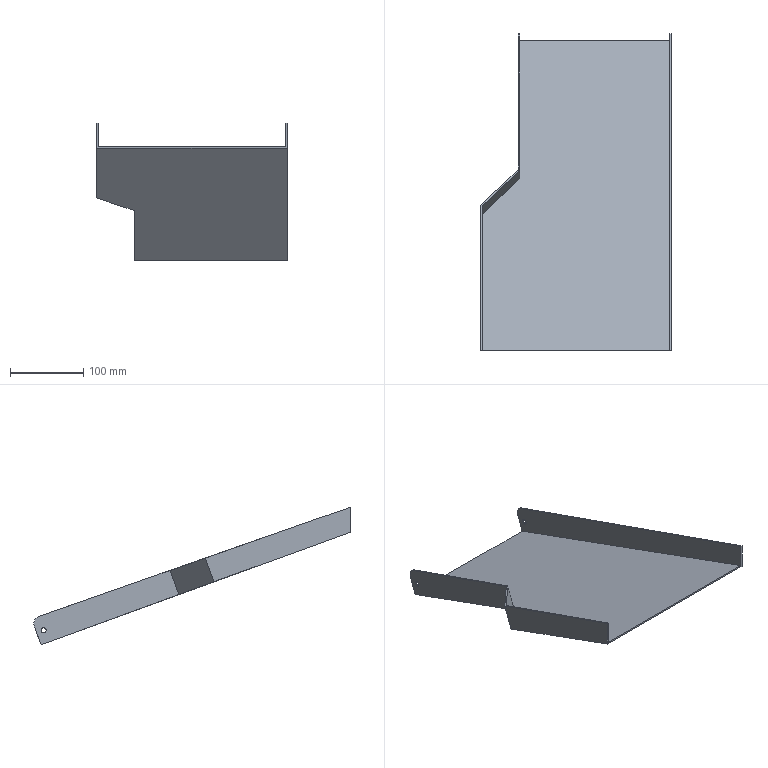Part | NX | features HB 2 | 1 solid | 18 faces | box 260 x 431.386 x 187.459 mm | volume 271044 mm3 | plane 14 | cylinder 4 | commonest cylinder face diameters 7 x2 20 x2
STEP:
#1=CARTESIAN_POINT('',(3672.,269.,-204.418));
#2=VERTEX_POINT('',#1);
#3=CARTESIAN_POINT('',(3672.,269.,-236.344));
#4=VERTEX_POINT('',#3);
#5=CARTESIAN_POINT('',(3672.,269.,-276.603));
#6=DIRECTION('',(0.,0.,-1.));
#7=VECTOR('',#6,1000.);
#8=LINE('',#5,#7);
#9=EDGE_CURVE('',#2,#4,#8,.T.);
#10=ORIENTED_EDGE('',*,*,#9,.F.);
#11=CARTESIAN_POINT('',(3670.,269.,-204.418));
#12=VERTEX_POINT('',#11);
#13=CARTESIAN_POINT('',(3603.,269.,-204.418));
#14=DIRECTION('',(-1.,0.,0.));
#15=VECTOR('',#14,1000.);
#16=LINE('',#13,#15);
#17=EDGE_CURVE('',#2,#12,#16,.T.);
#18=ORIENTED_EDGE('',*,*,#17,.T.);
#19=CARTESIAN_POINT('',(3670.,269.,-238.472));
#20=VERTEX_POINT('',#19);
#21=CARTESIAN_POINT('',(3670.,269.,-276.603));
#22=DIRECTION('',(0.,0.,-1.));
#23=VECTOR('',#22,1000.);
#24=LINE('',#21,#23);
#25=EDGE_CURVE('',#12,#20,#24,.T.);
#26=ORIENTED_EDGE('',*,*,#25,.T.);
#27=CARTESIAN_POINT('',(3930.,269.,-238.472));
#28=VERTEX_POINT('',#27);
#29=CARTESIAN_POINT('',(3698.,269.,-238.472));
#30=DIRECTION('',(1.,0.,0.));
#31=VECTOR('',#30,1000.);
#32=LINE('',#29,#31);
#33=EDGE_CURVE('',#20,#28,#32,.T.);
#34=ORIENTED_EDGE('',*,*,#33,.T.);
#35=CARTESIAN_POINT('',(3930.,269.,-204.418));
#36=VERTEX_POINT('',#35);
#37=CARTESIAN_POINT('',(3930.,269.,-276.603));
#38=DIRECTION('',(0.,0.,1.));
#39=VECTOR('',#38,1000.);
#40=LINE('',#37,#39);
#41=EDGE_CURVE('',#28,#36,#40,.T.);
#42=ORIENTED_EDGE('',*,*,#41,.T.);
#43=CARTESIAN_POINT('',(3928.,269.,-204.418));
#44=VERTEX_POINT('',#43);
#45=CARTESIAN_POINT('',(3930.,269.,-204.418));
#46=DIRECTION('',(-1.,0.,0.));
#47=VECTOR('',#46,1000.);
#48=LINE('',#45,#47);
#49=EDGE_CURVE('',#36,#44,#48,.T.);
#50=ORIENTED_EDGE('',*,*,#49,.T.);
#51=CARTESIAN_POINT('',(3928.,269.,-236.344));
#52=VERTEX_POINT('',#51);
#53=CARTESIAN_POINT('',(3928.,269.,-276.603));
#54=DIRECTION('',(0.,0.,1.));
#55=VECTOR('',#54,1000.);
#56=LINE('',#53,#55);
#57=EDGE_CURVE('',#52,#44,#56,.T.);
#58=ORIENTED_EDGE('',*,*,#57,.F.);
#59=CARTESIAN_POINT('',(3698.,269.,-236.344));
#60=DIRECTION('',(1.,0.,0.));
#61=VECTOR('',#60,1000.);
#62=LINE('',#59,#61);
#63=EDGE_CURVE('',#4,#52,#62,.T.);
#64=ORIENTED_EDGE('',*,*,#63,.F.);
#65=EDGE_LOOP('',(#10,#18,#26,#34,#42,#50,#58,#64));
#66=FACE_BOUND('',#65,.T.);
#67=CARTESIAN_POINT('',(4322.,269.,100.));
#68=DIRECTION('',(0.,-1.,0.));
#69=DIRECTION('',(0.,0.,1.));
#70=AXIS2_PLACEMENT_3D('',#67,#68,#69);
#71=PLANE('',#70);
#72=ADVANCED_FACE('',(#66),#71,.T.);
#73=CARTESIAN_POINT('',(3723.,502.577,-321.359));
#74=VERTEX_POINT('',#73);
#75=CARTESIAN_POINT('',(3672.,454.652,-303.916));
#76=VERTEX_POINT('',#75);
#77=CARTESIAN_POINT('',(3645.071,429.348,-294.705));
#78=DIRECTION('',(-0.7071,-0.6645,0.2418));
#79=VECTOR('',#78,1000.);
#80=LINE('',#77,#79);
#81=EDGE_CURVE('',#74,#76,#80,.T.);
#82=ORIENTED_EDGE('',*,*,#81,.T.);
#83=CARTESIAN_POINT('',(3672.,379.611,-276.603));
#84=DIRECTION('',(0.,-0.9397,0.342));
#85=VECTOR('',#84,1000.);
#86=LINE('',#83,#85);
#87=EDGE_CURVE('',#76,#4,#86,.T.);
#88=ORIENTED_EDGE('',*,*,#87,.T.);
#89=ORIENTED_EDGE('',*,*,#63,.T.);
#90=CARTESIAN_POINT('',(3928.,691.161,-389.998));
#91=VERTEX_POINT('',#90);
#92=CARTESIAN_POINT('',(3928.,379.611,-276.603));
#93=DIRECTION('',(0.,0.9397,-0.342));
#94=VECTOR('',#93,1000.);
#95=LINE('',#92,#94);
#96=EDGE_CURVE('',#52,#91,#95,.T.);
#97=ORIENTED_EDGE('',*,*,#96,.T.);
#98=CARTESIAN_POINT('',(3723.,691.161,-389.998));
#99=VERTEX_POINT('',#98);
#100=CARTESIAN_POINT('',(3698.,691.161,-389.998));
#101=DIRECTION('',(1.,0.,0.));
#102=VECTOR('',#101,1000.);
#103=LINE('',#100,#102);
#104=EDGE_CURVE('',#99,#91,#103,.T.);
#105=ORIENTED_EDGE('',*,*,#104,.F.);
#106=CARTESIAN_POINT('',(3723.,379.611,-276.603));
#107=DIRECTION('',(0.,-0.9397,0.342));
#108=VECTOR('',#107,1000.);
#109=LINE('',#106,#108);
#110=EDGE_CURVE('',#99,#74,#109,.T.);
#111=ORIENTED_EDGE('',*,*,#110,.T.);
#112=EDGE_LOOP('',(#82,#88,#89,#97,#105,#111));
#113=FACE_BOUND('',#112,.T.);
#114=CARTESIAN_POINT('',(3698.,379.611,-276.603));
#115=DIRECTION('',(0.,0.342,0.9397));
#116=DIRECTION('',(1.,0.,0.));
#117=AXIS2_PLACEMENT_3D('',#114,#115,#116);
#118=PLANE('',#117);
#119=ADVANCED_FACE('',(#113),#118,.T.);
#120=CARTESIAN_POINT('',(3672.,465.738,-273.457));
#121=VERTEX_POINT('',#120);
#122=CARTESIAN_POINT('',(3672.,454.652,-303.916));
#123=DIRECTION('',(0.,-0.342,-0.9397));
#124=VECTOR('',#123,1000.);
#125=LINE('',#122,#124);
#126=EDGE_CURVE('',#121,#76,#125,.T.);
#127=ORIENTED_EDGE('',*,*,#126,.F.);
#128=CARTESIAN_POINT('',(3672.,390.365,-247.007));
#129=DIRECTION('',(0.,-0.9436,0.3311));
#130=VECTOR('',#129,1000.);
#131=LINE('',#128,#130);
#132=EDGE_CURVE('',#121,#2,#131,.T.);
#133=ORIENTED_EDGE('',*,*,#132,.T.);
#134=ORIENTED_EDGE('',*,*,#9,.T.);
#135=ORIENTED_EDGE('',*,*,#87,.F.);
#136=EDGE_LOOP('',(#127,#133,#134,#135));
#137=FACE_BOUND('',#136,.T.);
#138=CARTESIAN_POINT('',(3672.,379.611,-276.603));
#139=DIRECTION('',(1.,0.,0.));
#140=DIRECTION('',(0.,-0.08716,0.9962));
#141=AXIS2_PLACEMENT_3D('',#138,#139,#140);
#142=PLANE('',#141);
#143=ADVANCED_FACE('',(#137),#142,.T.);
#144=CARTESIAN_POINT('',(3930.,693.697,-353.452));
#145=VERTEX_POINT('',#144);
#146=CARTESIAN_POINT('',(3930.,390.365,-247.007));
#147=DIRECTION('',(0.,-0.9436,0.3311));
#148=VECTOR('',#147,1000.);
#149=LINE('',#146,#148);
#150=EDGE_CURVE('',#145,#36,#149,.T.);
#151=ORIENTED_EDGE('',*,*,#150,.T.);
#152=ORIENTED_EDGE('',*,*,#41,.F.);
#153=CARTESIAN_POINT('',(3930.,690.477,-391.877));
#154=VERTEX_POINT('',#153);
#155=CARTESIAN_POINT('',(3930.,378.927,-278.482));
#156=DIRECTION('',(0.,-0.9397,0.342));
#157=VECTOR('',#156,1000.);
#158=LINE('',#155,#157);
#159=EDGE_CURVE('',#154,#28,#158,.T.);
#160=ORIENTED_EDGE('',*,*,#159,.F.);
#161=CARTESIAN_POINT('',(3930.,699.783,-366.309));
#162=VERTEX_POINT('',#161);
#163=CARTESIAN_POINT('',(3930.,692.943,-385.102));
#164=DIRECTION('',(0.,0.342,0.9397));
#165=VECTOR('',#164,1000.);
#166=LINE('',#163,#165);
#167=EDGE_CURVE('',#154,#162,#166,.T.);
#168=ORIENTED_EDGE('',*,*,#167,.T.);
#169=CARTESIAN_POINT('',(3930.,690.386,-362.888));
#170=DIRECTION('',(-1.,0.,0.));
#171=DIRECTION('',(0.,0.,1.));
#172=AXIS2_PLACEMENT_3D('',#169,#170,#171);
#173=CIRCLE('',#172,10.);
#174=EDGE_CURVE('',#145,#162,#173,.T.);
#175=ORIENTED_EDGE('',*,*,#174,.F.);
#176=EDGE_LOOP('',(#151,#152,#160,#168,#175));
#177=FACE_BOUND('',#176,.T.);
#178=CARTESIAN_POINT('',(3930.,686.966,-368.785));
#179=VERTEX_POINT('',#178);
#180=CARTESIAN_POINT('',(3930.,686.966,-372.285));
#181=DIRECTION('',(1.,0.,0.));
#182=DIRECTION('',(0.,0.,1.));
#183=AXIS2_PLACEMENT_3D('',#180,#181,#182);
#184=CIRCLE('',#183,3.5);
#185=EDGE_CURVE('',#179,#179,#184,.T.);
#186=ORIENTED_EDGE('',*,*,#185,.F.);
#187=EDGE_LOOP('',(#186));
#188=FACE_BOUND('',#187,.T.);
#189=CARTESIAN_POINT('',(3930.,379.611,-276.603));
#190=DIRECTION('',(-1.,0.,0.));
#191=DIRECTION('',(0.,-0.08716,0.9962));
#192=AXIS2_PLACEMENT_3D('',#189,#190,#191);
#193=PLANE('',#192);
#194=ADVANCED_FACE('',(#177,#188),#193,.F.);
#195=CARTESIAN_POINT('',(3928.,693.697,-353.452));
#196=VERTEX_POINT('',#195);
#197=CARTESIAN_POINT('',(3928.,390.365,-247.007));
#198=DIRECTION('',(0.,-0.9436,0.3311));
#199=VECTOR('',#198,1000.);
#200=LINE('',#197,#199);
#201=EDGE_CURVE('',#196,#44,#200,.T.);
#202=ORIENTED_EDGE('',*,*,#201,.T.);
#203=ORIENTED_EDGE('',*,*,#49,.F.);
#204=ORIENTED_EDGE('',*,*,#150,.F.);
#205=CARTESIAN_POINT('',(3930.,693.697,-353.452));
#206=DIRECTION('',(1.,0.,0.));
#207=VECTOR('',#206,1000.);
#208=LINE('',#205,#207);
#209=EDGE_CURVE('',#196,#145,#208,.T.);
#210=ORIENTED_EDGE('',*,*,#209,.F.);
#211=EDGE_LOOP('',(#202,#203,#204,#210));
#212=FACE_BOUND('',#211,.T.);
#213=CARTESIAN_POINT('',(3930.,390.365,-247.007));
#214=DIRECTION('',(0.,-0.3311,-0.9436));
#215=DIRECTION('',(0.,0.9436,-0.3311));
#216=AXIS2_PLACEMENT_3D('',#213,#214,#215);
#217=PLANE('',#216);
#218=ADVANCED_FACE('',(#212),#217,.F.);
#219=CARTESIAN_POINT('',(3721.,502.671,-323.521));
#220=VERTEX_POINT('',#219);
#221=CARTESIAN_POINT('',(3721.,690.477,-391.877));
#222=VERTEX_POINT('',#221);
#223=CARTESIAN_POINT('',(3721.,378.927,-278.482));
#224=DIRECTION('',(0.,0.9397,-0.342));
#225=VECTOR('',#224,1000.);
#226=LINE('',#223,#225);
#227=EDGE_CURVE('',#220,#222,#226,.T.);
#228=ORIENTED_EDGE('',*,*,#227,.T.);
#229=CARTESIAN_POINT('',(3698.,690.477,-391.877));
#230=DIRECTION('',(1.,0.,0.));
#231=VECTOR('',#230,1000.);
#232=LINE('',#229,#231);
#233=EDGE_CURVE('',#222,#154,#232,.T.);
#234=ORIENTED_EDGE('',*,*,#233,.T.);
#235=ORIENTED_EDGE('',*,*,#159,.T.);
#236=ORIENTED_EDGE('',*,*,#33,.F.);
#237=CARTESIAN_POINT('',(3670.,454.747,-306.078));
#238=VERTEX_POINT('',#237);
#239=CARTESIAN_POINT('',(3670.,378.927,-278.482));
#240=DIRECTION('',(0.,0.9397,-0.342));
#241=VECTOR('',#240,1000.);
#242=LINE('',#239,#241);
#243=EDGE_CURVE('',#20,#238,#242,.T.);
#244=ORIENTED_EDGE('',*,*,#243,.T.);
#245=CARTESIAN_POINT('',(3643.657,429.993,-297.069));
#246=DIRECTION('',(-0.7071,-0.6645,0.2418));
#247=VECTOR('',#246,1000.);
#248=LINE('',#245,#247);
#249=EDGE_CURVE('',#220,#238,#248,.T.);
#250=ORIENTED_EDGE('',*,*,#249,.F.);
#251=EDGE_LOOP('',(#228,#234,#235,#236,#244,#250));
#252=FACE_BOUND('',#251,.T.);
#253=CARTESIAN_POINT('',(3698.,378.927,-278.482));
#254=DIRECTION('',(0.,0.342,0.9397));
#255=DIRECTION('',(1.,0.,0.));
#256=AXIS2_PLACEMENT_3D('',#253,#254,#255);
#257=PLANE('',#256);
#258=ADVANCED_FACE('',(#252),#257,.F.);
#259=ORIENTED_EDGE('',*,*,#243,.F.);
#260=ORIENTED_EDGE('',*,*,#25,.F.);
#261=CARTESIAN_POINT('',(3670.,466.52,-273.732));
#262=VERTEX_POINT('',#261);
#263=CARTESIAN_POINT('',(3670.,390.365,-247.007));
#264=DIRECTION('',(0.,-0.9436,0.3311));
#265=VECTOR('',#264,1000.);
#266=LINE('',#263,#265);
#267=EDGE_CURVE('',#262,#12,#266,.T.);
#268=ORIENTED_EDGE('',*,*,#267,.F.);
#269=CARTESIAN_POINT('',(3670.,455.431,-304.199));
#270=DIRECTION('',(0.,-0.342,-0.9397));
#271=VECTOR('',#270,1000.);
#272=LINE('',#269,#271);
#273=EDGE_CURVE('',#262,#238,#272,.T.);
#274=ORIENTED_EDGE('',*,*,#273,.T.);
#275=EDGE_LOOP('',(#259,#260,#268,#274));
#276=FACE_BOUND('',#275,.T.);
#277=CARTESIAN_POINT('',(3670.,379.611,-276.603));
#278=DIRECTION('',(1.,0.,0.));
#279=DIRECTION('',(0.,0.08716,-0.9962));
#280=AXIS2_PLACEMENT_3D('',#277,#278,#279);
#281=PLANE('',#280);
#282=ADVANCED_FACE('',(#276),#281,.F.);
#283=CARTESIAN_POINT('',(3721.,514.646,-290.62));
#284=VERTEX_POINT('',#283);
#285=CARTESIAN_POINT('',(3670.986,467.45,-274.058));
#286=DIRECTION('',(0.7071,0.6672,-0.2341));
#287=VECTOR('',#286,1000.);
#288=LINE('',#285,#287);
#289=EDGE_CURVE('',#262,#284,#288,.T.);
#290=ORIENTED_EDGE('',*,*,#289,.F.);
#291=ORIENTED_EDGE('',*,*,#267,.T.);
#292=ORIENTED_EDGE('',*,*,#17,.F.);
#293=ORIENTED_EDGE('',*,*,#132,.F.);
#294=CARTESIAN_POINT('',(3723.,513.864,-290.346));
#295=VERTEX_POINT('',#294);
#296=CARTESIAN_POINT('',(3672.4,466.116,-273.59));
#297=DIRECTION('',(0.7071,0.6672,-0.2341));
#298=VECTOR('',#297,1000.);
#299=LINE('',#296,#298);
#300=EDGE_CURVE('',#121,#295,#299,.T.);
#301=ORIENTED_EDGE('',*,*,#300,.T.);
#302=CARTESIAN_POINT('',(3723.,693.697,-353.452));
#303=VERTEX_POINT('',#302);
#304=CARTESIAN_POINT('',(3723.,390.365,-247.007));
#305=DIRECTION('',(0.,-0.9436,0.3311));
#306=VECTOR('',#305,1000.);
#307=LINE('',#304,#306);
#308=EDGE_CURVE('',#303,#295,#307,.T.);
#309=ORIENTED_EDGE('',*,*,#308,.F.);
#310=CARTESIAN_POINT('',(3721.,693.697,-353.452));
#311=VERTEX_POINT('',#310);
#312=CARTESIAN_POINT('',(3698.,693.697,-353.452));
#313=DIRECTION('',(1.,0.,0.));
#314=VECTOR('',#313,1000.);
#315=LINE('',#312,#314);
#316=EDGE_CURVE('',#311,#303,#315,.T.);
#317=ORIENTED_EDGE('',*,*,#316,.F.);
#318=CARTESIAN_POINT('',(3721.,390.365,-247.007));
#319=DIRECTION('',(0.,-0.9436,0.3311));
#320=VECTOR('',#319,1000.);
#321=LINE('',#318,#320);
#322=EDGE_CURVE('',#311,#284,#321,.T.);
#323=ORIENTED_EDGE('',*,*,#322,.T.);
#324=EDGE_LOOP('',(#290,#291,#292,#293,#301,#309,#317,#323));
#325=FACE_BOUND('',#324,.T.);
#326=CARTESIAN_POINT('',(3603.,390.365,-247.007));
#327=DIRECTION('',(0.,-0.3311,-0.9436));
#328=DIRECTION('',(0.,0.9436,-0.3311));
#329=AXIS2_PLACEMENT_3D('',#326,#327,#328);
#330=PLANE('',#329);
#331=ADVANCED_FACE('',(#325),#330,.F.);
#332=ORIENTED_EDGE('',*,*,#96,.F.);
#333=ORIENTED_EDGE('',*,*,#57,.T.);
#334=ORIENTED_EDGE('',*,*,#201,.F.);
#335=CARTESIAN_POINT('',(3928.,699.783,-366.309));
#336=VERTEX_POINT('',#335);
#337=CARTESIAN_POINT('',(3928.,690.386,-362.888));
#338=DIRECTION('',(1.,0.,0.));
#339=DIRECTION('',(0.,0.,1.));
#340=AXIS2_PLACEMENT_3D('',#337,#338,#339);
#341=CIRCLE('',#340,10.);
#342=EDGE_CURVE('',#336,#196,#341,.T.);
#343=ORIENTED_EDGE('',*,*,#342,.F.);
#344=CARTESIAN_POINT('',(3928.,692.943,-385.102));
#345=DIRECTION('',(0.,0.342,0.9397));
#346=VECTOR('',#345,1000.);
#347=LINE('',#344,#346);
#348=EDGE_CURVE('',#91,#336,#347,.T.);
#349=ORIENTED_EDGE('',*,*,#348,.F.);
#350=EDGE_LOOP('',(#332,#333,#334,#343,#349));
#351=FACE_BOUND('',#350,.T.);
#352=CARTESIAN_POINT('',(3928.,686.966,-368.785));
#353=VERTEX_POINT('',#352);
#354=CARTESIAN_POINT('',(3928.,686.966,-372.285));
#355=DIRECTION('',(-1.,0.,0.));
#356=DIRECTION('',(0.,0.,1.));
#357=AXIS2_PLACEMENT_3D('',#354,#355,#356);
#358=CIRCLE('',#357,3.5);
#359=EDGE_CURVE('',#353,#353,#358,.T.);
#360=ORIENTED_EDGE('',*,*,#359,.F.);
#361=EDGE_LOOP('',(#360));
#362=FACE_BOUND('',#361,.T.);
#363=CARTESIAN_POINT('',(3928.,379.611,-276.603));
#364=DIRECTION('',(-1.,0.,0.));
#365=DIRECTION('',(0.,-0.08716,0.9962));
#366=AXIS2_PLACEMENT_3D('',#363,#364,#365);
#367=PLANE('',#366);
#368=ADVANCED_FACE('',(#351,#362),#367,.T.);
#369=CARTESIAN_POINT('',(3723.,686.661,-368.799));
#370=VERTEX_POINT('',#369);
#371=CARTESIAN_POINT('',(3723.,686.966,-372.285));
#372=DIRECTION('',(1.,0.,0.));
#373=DIRECTION('',(0.,-0.08716,0.9962));
#374=AXIS2_PLACEMENT_3D('',#371,#372,#373);
#375=CIRCLE('',#374,3.5);
#376=EDGE_CURVE('',#370,#370,#375,.T.);
#377=ORIENTED_EDGE('',*,*,#376,.F.);
#378=EDGE_LOOP('',(#377));
#379=FACE_BOUND('',#378,.T.);
#380=ORIENTED_EDGE('',*,*,#110,.F.);
#381=CARTESIAN_POINT('',(3723.,699.783,-366.309));
#382=VERTEX_POINT('',#381);
#383=CARTESIAN_POINT('',(3723.,692.943,-385.102));
#384=DIRECTION('',(0.,0.342,0.9397));
#385=VECTOR('',#384,1000.);
#386=LINE('',#383,#385);
#387=EDGE_CURVE('',#99,#382,#386,.T.);
#388=ORIENTED_EDGE('',*,*,#387,.T.);
#389=CARTESIAN_POINT('',(3723.,690.386,-362.888));
#390=DIRECTION('',(-1.,0.,0.));
#391=DIRECTION('',(0.,0.,-1.));
#392=AXIS2_PLACEMENT_3D('',#389,#390,#391);
#393=CIRCLE('',#392,10.);
#394=EDGE_CURVE('',#303,#382,#393,.T.);
#395=ORIENTED_EDGE('',*,*,#394,.F.);
#396=ORIENTED_EDGE('',*,*,#308,.T.);
#397=CARTESIAN_POINT('',(3723.,512.837,-293.168));
#398=DIRECTION('',(0.,0.342,0.9397));
#399=VECTOR('',#398,1000.);
#400=LINE('',#397,#399);
#401=EDGE_CURVE('',#74,#295,#400,.T.);
#402=ORIENTED_EDGE('',*,*,#401,.F.);
#403=EDGE_LOOP('',(#380,#388,#395,#396,#402));
#404=FACE_BOUND('',#403,.T.);
#405=CARTESIAN_POINT('',(3723.,379.611,-276.603));
#406=DIRECTION('',(1.,0.,0.));
#407=DIRECTION('',(0.,-0.08716,0.9962));
#408=AXIS2_PLACEMENT_3D('',#405,#406,#407);
#409=PLANE('',#408);
#410=ADVANCED_FACE('',(#379,#404),#409,.T.);
#411=CARTESIAN_POINT('',(3721.,686.661,-368.799));
#412=VERTEX_POINT('',#411);
#413=CARTESIAN_POINT('',(3721.,686.966,-372.285));
#414=DIRECTION('',(1.,0.,0.));
#415=DIRECTION('',(0.,-0.08716,0.9962));
#416=AXIS2_PLACEMENT_3D('',#413,#414,#415);
#417=CIRCLE('',#416,3.5);
#418=EDGE_CURVE('',#412,#412,#417,.T.);
#419=ORIENTED_EDGE('',*,*,#418,.T.);
#420=EDGE_LOOP('',(#419));
#421=FACE_BOUND('',#420,.T.);
#422=CARTESIAN_POINT('',(3721.,513.616,-293.451));
#423=DIRECTION('',(0.,0.342,0.9397));
#424=VECTOR('',#423,1000.);
#425=LINE('',#422,#424);
#426=EDGE_CURVE('',#220,#284,#425,.T.);
#427=ORIENTED_EDGE('',*,*,#426,.T.);
#428=ORIENTED_EDGE('',*,*,#322,.F.);
#429=CARTESIAN_POINT('',(3721.,699.783,-366.309));
#430=VERTEX_POINT('',#429);
#431=CARTESIAN_POINT('',(3721.,690.386,-362.888));
#432=DIRECTION('',(1.,0.,0.));
#433=DIRECTION('',(0.,0.,-1.));
#434=AXIS2_PLACEMENT_3D('',#431,#432,#433);
#435=CIRCLE('',#434,10.);
#436=EDGE_CURVE('',#430,#311,#435,.T.);
#437=ORIENTED_EDGE('',*,*,#436,.F.);
#438=CARTESIAN_POINT('',(3721.,692.943,-385.102));
#439=DIRECTION('',(0.,0.342,0.9397));
#440=VECTOR('',#439,1000.);
#441=LINE('',#438,#440);
#442=EDGE_CURVE('',#222,#430,#441,.T.);
#443=ORIENTED_EDGE('',*,*,#442,.F.);
#444=ORIENTED_EDGE('',*,*,#227,.F.);
#445=EDGE_LOOP('',(#427,#428,#437,#443,#444));
#446=FACE_BOUND('',#445,.T.);
#447=CARTESIAN_POINT('',(3721.,379.611,-276.603));
#448=DIRECTION('',(1.,0.,0.));
#449=DIRECTION('',(0.,0.08716,-0.9962));
#450=AXIS2_PLACEMENT_3D('',#447,#448,#449);
#451=PLANE('',#450);
#452=ADVANCED_FACE('',(#421,#446),#451,.F.);
#453=ORIENTED_EDGE('',*,*,#376,.T.);
#454=EDGE_LOOP('',(#453));
#455=FACE_BOUND('',#454,.T.);
#456=ORIENTED_EDGE('',*,*,#418,.F.);
#457=EDGE_LOOP('',(#456));
#458=FACE_BOUND('',#457,.T.);
#459=CARTESIAN_POINT('',(2999.,686.966,-372.285));
#460=DIRECTION('',(1.,0.,0.));
#461=DIRECTION('',(0.,0.08716,-0.9962));
#462=AXIS2_PLACEMENT_3D('',#459,#460,#461);
#463=CYLINDRICAL_SURFACE('',#462,3.5);
#464=ADVANCED_FACE('',(#455,#458),#463,.F.);
#465=ORIENTED_EDGE('',*,*,#394,.T.);
#466=CARTESIAN_POINT('',(3698.,699.783,-366.309));
#467=DIRECTION('',(-1.,0.,0.));
#468=VECTOR('',#467,1000.);
#469=LINE('',#466,#468);
#470=EDGE_CURVE('',#382,#430,#469,.T.);
#471=ORIENTED_EDGE('',*,*,#470,.T.);
#472=ORIENTED_EDGE('',*,*,#436,.T.);
#473=ORIENTED_EDGE('',*,*,#316,.T.);
#474=EDGE_LOOP('',(#465,#471,#472,#473));
#475=FACE_BOUND('',#474,.T.);
#476=CARTESIAN_POINT('',(3698.,690.386,-362.888));
#477=DIRECTION('',(1.,0.,0.));
#478=DIRECTION('',(0.,0.,1.));
#479=AXIS2_PLACEMENT_3D('',#476,#477,#478);
#480=CYLINDRICAL_SURFACE('',#479,10.);
#481=ADVANCED_FACE('',(#475),#480,.T.);
#482=ORIENTED_EDGE('',*,*,#104,.T.);
#483=ORIENTED_EDGE('',*,*,#348,.T.);
#484=CARTESIAN_POINT('',(3930.,699.783,-366.309));
#485=DIRECTION('',(-1.,0.,0.));
#486=VECTOR('',#485,1000.);
#487=LINE('',#484,#486);
#488=EDGE_CURVE('',#162,#336,#487,.T.);
#489=ORIENTED_EDGE('',*,*,#488,.F.);
#490=ORIENTED_EDGE('',*,*,#167,.F.);
#491=ORIENTED_EDGE('',*,*,#233,.F.);
#492=ORIENTED_EDGE('',*,*,#442,.T.);
#493=ORIENTED_EDGE('',*,*,#470,.F.);
#494=ORIENTED_EDGE('',*,*,#387,.F.);
#495=EDGE_LOOP('',(#482,#483,#489,#490,#491,#492,#493,#494));
#496=FACE_BOUND('',#495,.T.);
#497=CARTESIAN_POINT('',(3698.,692.943,-385.102));
#498=DIRECTION('',(0.,-0.9397,0.342));
#499=DIRECTION('',(0.,-0.342,-0.9397));
#500=AXIS2_PLACEMENT_3D('',#497,#498,#499);
#501=PLANE('',#500);
#502=ADVANCED_FACE('',(#496),#501,.F.);
#503=ORIENTED_EDGE('',*,*,#342,.T.);
#504=ORIENTED_EDGE('',*,*,#209,.T.);
#505=ORIENTED_EDGE('',*,*,#174,.T.);
#506=ORIENTED_EDGE('',*,*,#488,.T.);
#507=EDGE_LOOP('',(#503,#504,#505,#506));
#508=FACE_BOUND('',#507,.T.);
#509=CARTESIAN_POINT('',(3930.,690.386,-362.888));
#510=DIRECTION('',(-1.,0.,0.));
#511=DIRECTION('',(0.,0.,-1.));
#512=AXIS2_PLACEMENT_3D('',#509,#510,#511);
#513=CYLINDRICAL_SURFACE('',#512,10.);
#514=ADVANCED_FACE('',(#508),#513,.T.);
#515=ORIENTED_EDGE('',*,*,#359,.T.);
#516=EDGE_LOOP('',(#515));
#517=FACE_BOUND('',#516,.T.);
#518=ORIENTED_EDGE('',*,*,#185,.T.);
#519=EDGE_LOOP('',(#518));
#520=FACE_BOUND('',#519,.T.);
#521=CARTESIAN_POINT('',(3025.,686.966,-372.285));
#522=DIRECTION('',(1.,0.,0.));
#523=DIRECTION('',(0.,0.08716,-0.9962));
#524=AXIS2_PLACEMENT_3D('',#521,#522,#523);
#525=CYLINDRICAL_SURFACE('',#524,3.5);
#526=ADVANCED_FACE('',(#517,#520),#525,.F.);
#527=ORIENTED_EDGE('',*,*,#249,.T.);
#528=ORIENTED_EDGE('',*,*,#273,.F.);
#529=ORIENTED_EDGE('',*,*,#289,.T.);
#530=ORIENTED_EDGE('',*,*,#426,.F.);
#531=EDGE_LOOP('',(#527,#528,#529,#530));
#532=FACE_BOUND('',#531,.T.);
#533=CARTESIAN_POINT('',(3671.,466.631,-276.35));
#534=DIRECTION('',(-0.7071,0.6645,-0.2418));
#535=DIRECTION('',(0.,0.342,0.9397));
#536=AXIS2_PLACEMENT_3D('',#533,#534,#535);
#537=PLANE('',#536);
#538=ADVANCED_FACE('',(#532),#537,.T.);
#539=ORIENTED_EDGE('',*,*,#401,.T.);
#540=ORIENTED_EDGE('',*,*,#300,.F.);
#541=ORIENTED_EDGE('',*,*,#126,.T.);
#542=ORIENTED_EDGE('',*,*,#81,.F.);
#543=EDGE_LOOP('',(#539,#540,#541,#542));
#544=FACE_BOUND('',#543,.T.);
#545=CARTESIAN_POINT('',(3672.414,465.302,-275.866));
#546=DIRECTION('',(-0.7071,0.6645,-0.2418));
#547=DIRECTION('',(0.,0.342,0.9397));
#548=AXIS2_PLACEMENT_3D('',#545,#546,#547);
#549=PLANE('',#548);
#550=ADVANCED_FACE('',(#544),#549,.F.);
#551=CLOSED_SHELL('',(#72,#119,#143,#194,#218,#258,#282,#331,#368,#410,#452,#464,#481,#502,#514,#526,#538,#550));
#552=MANIFOLD_SOLID_BREP('',#551);
#553=(LENGTH_UNIT()NAMED_UNIT(*)SI_UNIT(.MILLI.,.METRE.));
#554=UNCERTAINTY_MEASURE_WITH_UNIT(LENGTH_MEASURE(0.00001),#553,'','');
#555=(NAMED_UNIT(*)PLANE_ANGLE_UNIT()SI_UNIT($,.RADIAN.));
#556=(NAMED_UNIT(*)SI_UNIT($,.STERADIAN.)SOLID_ANGLE_UNIT());
#557=(GEOMETRIC_REPRESENTATION_CONTEXT(3)GLOBAL_UNCERTAINTY_ASSIGNED_CONTEXT((#554))GLOBAL_UNIT_ASSIGNED_CONTEXT((#553,#555,#556))REPRESENTATION_CONTEXT('',''));
#558=ADVANCED_BREP_SHAPE_REPRESENTATION('',(#552),#557);